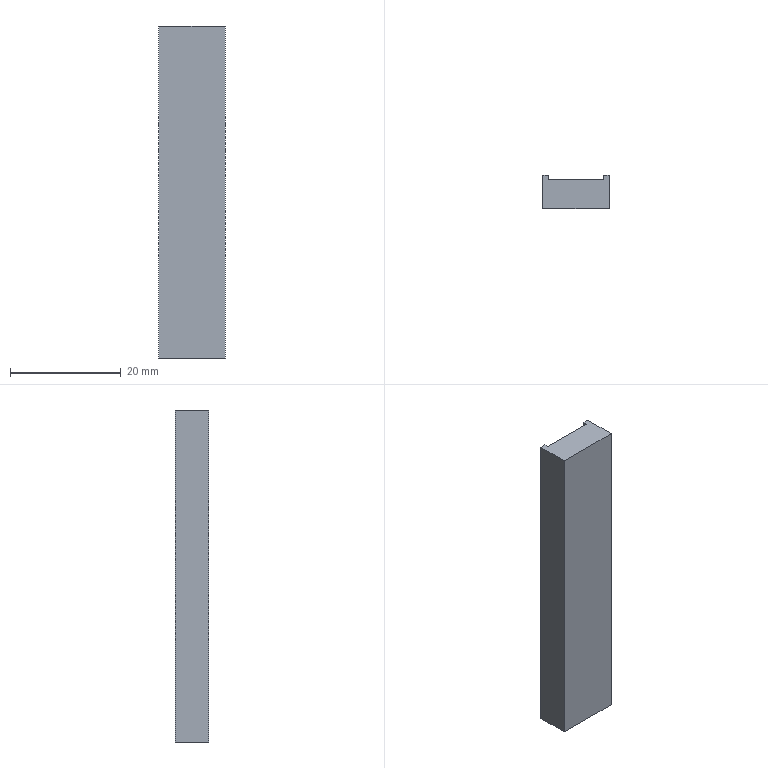Part | SolidWorks | features Extrusion 1, ICE 1 | 1 solid | 10 faces | box 12 x 6 x 60 mm | volume 3870 mm3 | plane 10
STEP:
#1=CARTESIAN_POINT('',(-5.,6.,-30.));
#2=VERTEX_POINT('',#1);
#3=CARTESIAN_POINT('',(-5.,6.,30.));
#4=VERTEX_POINT('',#3);
#5=CARTESIAN_POINT('',(-5.,6.,30.));
#6=DIRECTION('',(0.,0.,1.));
#7=VECTOR('',#6,1000.);
#8=LINE('',#5,#7);
#9=EDGE_CURVE('',#2,#4,#8,.T.);
#10=ORIENTED_EDGE('',*,*,#9,.F.);
#11=CARTESIAN_POINT('',(-6.,6.,-30.));
#12=VERTEX_POINT('',#11);
#13=CARTESIAN_POINT('',(6.,6.,-30.));
#14=DIRECTION('',(-1.,0.,0.));
#15=VECTOR('',#14,1000.);
#16=LINE('',#13,#15);
#17=EDGE_CURVE('',#2,#12,#16,.T.);
#18=ORIENTED_EDGE('',*,*,#17,.T.);
#19=CARTESIAN_POINT('',(-6.,6.,30.));
#20=VERTEX_POINT('',#19);
#21=CARTESIAN_POINT('',(-6.,6.,30.));
#22=DIRECTION('',(0.,0.,1.));
#23=VECTOR('',#22,1000.);
#24=LINE('',#21,#23);
#25=EDGE_CURVE('',#12,#20,#24,.T.);
#26=ORIENTED_EDGE('',*,*,#25,.T.);
#27=CARTESIAN_POINT('',(6.,6.,30.));
#28=DIRECTION('',(1.,0.,0.));
#29=VECTOR('',#28,1000.);
#30=LINE('',#27,#29);
#31=EDGE_CURVE('',#20,#4,#30,.T.);
#32=ORIENTED_EDGE('',*,*,#31,.T.);
#33=EDGE_LOOP('',(#10,#18,#26,#32));
#34=FACE_OUTER_BOUND('',#33,.T.);
#35=CARTESIAN_POINT('',(0.,6.,0.));
#36=DIRECTION('',(0.,1.,0.));
#37=DIRECTION('',(0.,0.,1.));
#38=AXIS2_PLACEMENT_3D('',#35,#36,#37);
#39=PLANE('',#38);
#40=ADVANCED_FACE('',(#34),#39,.T.);
#41=CARTESIAN_POINT('',(-6.,0.,-30.));
#42=VERTEX_POINT('',#41);
#43=CARTESIAN_POINT('',(-6.,0.,30.));
#44=VERTEX_POINT('',#43);
#45=CARTESIAN_POINT('',(-6.,0.,30.));
#46=DIRECTION('',(0.,0.,1.));
#47=VECTOR('',#46,1000.);
#48=LINE('',#45,#47);
#49=EDGE_CURVE('',#42,#44,#48,.T.);
#50=ORIENTED_EDGE('',*,*,#49,.T.);
#51=CARTESIAN_POINT('',(-6.,6.,30.));
#52=DIRECTION('',(0.,-1.,0.));
#53=VECTOR('',#52,1000.);
#54=LINE('',#51,#53);
#55=EDGE_CURVE('',#20,#44,#54,.T.);
#56=ORIENTED_EDGE('',*,*,#55,.F.);
#57=ORIENTED_EDGE('',*,*,#25,.F.);
#58=CARTESIAN_POINT('',(-6.,6.,-30.));
#59=DIRECTION('',(0.,-1.,0.));
#60=VECTOR('',#59,1000.);
#61=LINE('',#58,#60);
#62=EDGE_CURVE('',#12,#42,#61,.T.);
#63=ORIENTED_EDGE('',*,*,#62,.T.);
#64=EDGE_LOOP('',(#50,#56,#57,#63));
#65=FACE_OUTER_BOUND('',#64,.T.);
#66=CARTESIAN_POINT('',(-6.,6.,30.));
#67=DIRECTION('',(1.,0.,0.));
#68=DIRECTION('',(0.,0.,-1.));
#69=AXIS2_PLACEMENT_3D('',#66,#67,#68);
#70=PLANE('',#69);
#71=ADVANCED_FACE('',(#65),#70,.F.);
#72=CARTESIAN_POINT('',(-5.,5.25,30.));
#73=VERTEX_POINT('',#72);
#74=CARTESIAN_POINT('',(5.,5.25,30.));
#75=VERTEX_POINT('',#74);
#76=CARTESIAN_POINT('',(5.,5.25,30.));
#77=DIRECTION('',(1.,0.,0.));
#78=VECTOR('',#77,1000.);
#79=LINE('',#76,#78);
#80=EDGE_CURVE('',#73,#75,#79,.T.);
#81=ORIENTED_EDGE('',*,*,#80,.F.);
#82=CARTESIAN_POINT('',(-5.,5.25,30.));
#83=DIRECTION('',(0.,1.,0.));
#84=VECTOR('',#83,1000.);
#85=LINE('',#82,#84);
#86=EDGE_CURVE('',#73,#4,#85,.T.);
#87=ORIENTED_EDGE('',*,*,#86,.T.);
#88=ORIENTED_EDGE('',*,*,#31,.F.);
#89=ORIENTED_EDGE('',*,*,#55,.T.);
#90=CARTESIAN_POINT('',(6.,0.,30.));
#91=VERTEX_POINT('',#90);
#92=CARTESIAN_POINT('',(6.,0.,30.));
#93=DIRECTION('',(1.,0.,0.));
#94=VECTOR('',#93,1000.);
#95=LINE('',#92,#94);
#96=EDGE_CURVE('',#44,#91,#95,.T.);
#97=ORIENTED_EDGE('',*,*,#96,.T.);
#98=CARTESIAN_POINT('',(6.,6.,30.));
#99=VERTEX_POINT('',#98);
#100=CARTESIAN_POINT('',(6.,6.,30.));
#101=DIRECTION('',(0.,-1.,0.));
#102=VECTOR('',#101,1000.);
#103=LINE('',#100,#102);
#104=EDGE_CURVE('',#99,#91,#103,.T.);
#105=ORIENTED_EDGE('',*,*,#104,.F.);
#106=CARTESIAN_POINT('',(5.,6.,30.));
#107=VERTEX_POINT('',#106);
#108=CARTESIAN_POINT('',(6.,6.,30.));
#109=DIRECTION('',(1.,0.,0.));
#110=VECTOR('',#109,1000.);
#111=LINE('',#108,#110);
#112=EDGE_CURVE('',#107,#99,#111,.T.);
#113=ORIENTED_EDGE('',*,*,#112,.F.);
#114=CARTESIAN_POINT('',(5.,5.25,30.));
#115=DIRECTION('',(0.,1.,0.));
#116=VECTOR('',#115,1000.);
#117=LINE('',#114,#116);
#118=EDGE_CURVE('',#75,#107,#117,.T.);
#119=ORIENTED_EDGE('',*,*,#118,.F.);
#120=EDGE_LOOP('',(#81,#87,#88,#89,#97,#105,#113,#119));
#121=FACE_OUTER_BOUND('',#120,.T.);
#122=CARTESIAN_POINT('',(6.,6.,30.));
#123=DIRECTION('',(0.,0.,-1.));
#124=DIRECTION('',(-1.,0.,0.));
#125=AXIS2_PLACEMENT_3D('',#122,#123,#124);
#126=PLANE('',#125);
#127=ADVANCED_FACE('',(#121),#126,.F.);
#128=CARTESIAN_POINT('',(6.,0.,-30.));
#129=VERTEX_POINT('',#128);
#130=CARTESIAN_POINT('',(6.,0.,30.));
#131=DIRECTION('',(0.,0.,-1.));
#132=VECTOR('',#131,1000.);
#133=LINE('',#130,#132);
#134=EDGE_CURVE('',#91,#129,#133,.T.);
#135=ORIENTED_EDGE('',*,*,#134,.T.);
#136=CARTESIAN_POINT('',(6.,6.,-30.));
#137=VERTEX_POINT('',#136);
#138=CARTESIAN_POINT('',(6.,6.,-30.));
#139=DIRECTION('',(0.,-1.,0.));
#140=VECTOR('',#139,1000.);
#141=LINE('',#138,#140);
#142=EDGE_CURVE('',#137,#129,#141,.T.);
#143=ORIENTED_EDGE('',*,*,#142,.F.);
#144=CARTESIAN_POINT('',(6.,6.,30.));
#145=DIRECTION('',(0.,0.,-1.));
#146=VECTOR('',#145,1000.);
#147=LINE('',#144,#146);
#148=EDGE_CURVE('',#99,#137,#147,.T.);
#149=ORIENTED_EDGE('',*,*,#148,.F.);
#150=ORIENTED_EDGE('',*,*,#104,.T.);
#151=EDGE_LOOP('',(#135,#143,#149,#150));
#152=FACE_OUTER_BOUND('',#151,.T.);
#153=CARTESIAN_POINT('',(6.,6.,30.));
#154=DIRECTION('',(-1.,0.,0.));
#155=DIRECTION('',(0.,0.,1.));
#156=AXIS2_PLACEMENT_3D('',#153,#154,#155);
#157=PLANE('',#156);
#158=ADVANCED_FACE('',(#152),#157,.F.);
#159=ORIENTED_EDGE('',*,*,#17,.F.);
#160=CARTESIAN_POINT('',(-5.,5.25,-30.));
#161=VERTEX_POINT('',#160);
#162=CARTESIAN_POINT('',(-5.,5.25,-30.));
#163=DIRECTION('',(0.,1.,0.));
#164=VECTOR('',#163,1000.);
#165=LINE('',#162,#164);
#166=EDGE_CURVE('',#161,#2,#165,.T.);
#167=ORIENTED_EDGE('',*,*,#166,.F.);
#168=CARTESIAN_POINT('',(5.,5.25,-30.));
#169=VERTEX_POINT('',#168);
#170=CARTESIAN_POINT('',(5.,5.25,-30.));
#171=DIRECTION('',(-1.,0.,0.));
#172=VECTOR('',#171,1000.);
#173=LINE('',#170,#172);
#174=EDGE_CURVE('',#169,#161,#173,.T.);
#175=ORIENTED_EDGE('',*,*,#174,.F.);
#176=CARTESIAN_POINT('',(5.,6.,-30.));
#177=VERTEX_POINT('',#176);
#178=CARTESIAN_POINT('',(5.,5.25,-30.));
#179=DIRECTION('',(0.,1.,0.));
#180=VECTOR('',#179,1000.);
#181=LINE('',#178,#180);
#182=EDGE_CURVE('',#169,#177,#181,.T.);
#183=ORIENTED_EDGE('',*,*,#182,.T.);
#184=CARTESIAN_POINT('',(6.,6.,-30.));
#185=DIRECTION('',(-1.,0.,0.));
#186=VECTOR('',#185,1000.);
#187=LINE('',#184,#186);
#188=EDGE_CURVE('',#137,#177,#187,.T.);
#189=ORIENTED_EDGE('',*,*,#188,.F.);
#190=ORIENTED_EDGE('',*,*,#142,.T.);
#191=CARTESIAN_POINT('',(6.,0.,-30.));
#192=DIRECTION('',(-1.,0.,0.));
#193=VECTOR('',#192,1000.);
#194=LINE('',#191,#193);
#195=EDGE_CURVE('',#129,#42,#194,.T.);
#196=ORIENTED_EDGE('',*,*,#195,.T.);
#197=ORIENTED_EDGE('',*,*,#62,.F.);
#198=EDGE_LOOP('',(#159,#167,#175,#183,#189,#190,#196,#197));
#199=FACE_OUTER_BOUND('',#198,.T.);
#200=CARTESIAN_POINT('',(6.,6.,-30.));
#201=DIRECTION('',(0.,0.,1.));
#202=DIRECTION('',(1.,0.,0.));
#203=AXIS2_PLACEMENT_3D('',#200,#201,#202);
#204=PLANE('',#203);
#205=ADVANCED_FACE('',(#199),#204,.F.);
#206=CARTESIAN_POINT('',(5.,6.,30.));
#207=DIRECTION('',(0.,0.,-1.));
#208=VECTOR('',#207,1000.);
#209=LINE('',#206,#208);
#210=EDGE_CURVE('',#107,#177,#209,.T.);
#211=ORIENTED_EDGE('',*,*,#210,.F.);
#212=ORIENTED_EDGE('',*,*,#112,.T.);
#213=ORIENTED_EDGE('',*,*,#148,.T.);
#214=ORIENTED_EDGE('',*,*,#188,.T.);
#215=EDGE_LOOP('',(#211,#212,#213,#214));
#216=FACE_OUTER_BOUND('',#215,.T.);
#217=CARTESIAN_POINT('',(0.,6.,0.));
#218=DIRECTION('',(0.,1.,0.));
#219=DIRECTION('',(0.,0.,1.));
#220=AXIS2_PLACEMENT_3D('',#217,#218,#219);
#221=PLANE('',#220);
#222=ADVANCED_FACE('',(#216),#221,.T.);
#223=ORIENTED_EDGE('',*,*,#49,.F.);
#224=ORIENTED_EDGE('',*,*,#195,.F.);
#225=ORIENTED_EDGE('',*,*,#134,.F.);
#226=ORIENTED_EDGE('',*,*,#96,.F.);
#227=EDGE_LOOP('',(#223,#224,#225,#226));
#228=FACE_OUTER_BOUND('',#227,.T.);
#229=CARTESIAN_POINT('',(0.,0.,0.));
#230=DIRECTION('',(0.,1.,0.));
#231=DIRECTION('',(0.,0.,1.));
#232=AXIS2_PLACEMENT_3D('',#229,#230,#231);
#233=PLANE('',#232);
#234=ADVANCED_FACE('',(#228),#233,.F.);
#235=ORIENTED_EDGE('',*,*,#9,.T.);
#236=ORIENTED_EDGE('',*,*,#86,.F.);
#237=CARTESIAN_POINT('',(-5.,5.25,30.));
#238=DIRECTION('',(0.,0.,1.));
#239=VECTOR('',#238,1000.);
#240=LINE('',#237,#239);
#241=EDGE_CURVE('',#161,#73,#240,.T.);
#242=ORIENTED_EDGE('',*,*,#241,.F.);
#243=ORIENTED_EDGE('',*,*,#166,.T.);
#244=EDGE_LOOP('',(#235,#236,#242,#243));
#245=FACE_OUTER_BOUND('',#244,.T.);
#246=CARTESIAN_POINT('',(-5.,5.25,30.));
#247=DIRECTION('',(-1.,0.,0.));
#248=DIRECTION('',(0.,0.,1.));
#249=AXIS2_PLACEMENT_3D('',#246,#247,#248);
#250=PLANE('',#249);
#251=ADVANCED_FACE('',(#245),#250,.F.);
#252=ORIENTED_EDGE('',*,*,#210,.T.);
#253=ORIENTED_EDGE('',*,*,#182,.F.);
#254=CARTESIAN_POINT('',(5.,5.25,30.));
#255=DIRECTION('',(0.,0.,-1.));
#256=VECTOR('',#255,1000.);
#257=LINE('',#254,#256);
#258=EDGE_CURVE('',#75,#169,#257,.T.);
#259=ORIENTED_EDGE('',*,*,#258,.F.);
#260=ORIENTED_EDGE('',*,*,#118,.T.);
#261=EDGE_LOOP('',(#252,#253,#259,#260));
#262=FACE_OUTER_BOUND('',#261,.T.);
#263=CARTESIAN_POINT('',(5.,5.25,30.));
#264=DIRECTION('',(1.,0.,0.));
#265=DIRECTION('',(0.,0.,-1.));
#266=AXIS2_PLACEMENT_3D('',#263,#264,#265);
#267=PLANE('',#266);
#268=ADVANCED_FACE('',(#262),#267,.F.);
#269=ORIENTED_EDGE('',*,*,#241,.T.);
#270=ORIENTED_EDGE('',*,*,#80,.T.);
#271=ORIENTED_EDGE('',*,*,#258,.T.);
#272=ORIENTED_EDGE('',*,*,#174,.T.);
#273=EDGE_LOOP('',(#269,#270,#271,#272));
#274=FACE_OUTER_BOUND('',#273,.T.);
#275=CARTESIAN_POINT('',(0.,5.25,0.));
#276=DIRECTION('',(0.,1.,0.));
#277=DIRECTION('',(0.,0.,1.));
#278=AXIS2_PLACEMENT_3D('',#275,#276,#277);
#279=PLANE('',#278);
#280=ADVANCED_FACE('',(#274),#279,.T.);
#281=CLOSED_SHELL('',(#40,#71,#127,#158,#205,#222,#234,#251,#268,#280));
#282=MANIFOLD_SOLID_BREP('',#281);
#283=CARTESIAN_POINT('',(0.,0.,0.));
#284=DIRECTION('',(0.,0.,1.));
#285=DIRECTION('',(1.,0.,0.));
#286=AXIS2_PLACEMENT_3D('',#283,#284,#285);
#287=(LENGTH_UNIT()NAMED_UNIT(*)SI_UNIT(.MILLI.,.METRE.));
#288=UNCERTAINTY_MEASURE_WITH_UNIT(LENGTH_MEASURE(0.00001),#287,'','');
#289=(NAMED_UNIT(*)PLANE_ANGLE_UNIT()SI_UNIT($,.RADIAN.));
#290=(NAMED_UNIT(*)SI_UNIT($,.STERADIAN.)SOLID_ANGLE_UNIT());
#291=(GEOMETRIC_REPRESENTATION_CONTEXT(3)GLOBAL_UNCERTAINTY_ASSIGNED_CONTEXT((#288))GLOBAL_UNIT_ASSIGNED_CONTEXT((#287,#289,#290))REPRESENTATION_CONTEXT('',''));
#292=ADVANCED_BREP_SHAPE_REPRESENTATION('',(#282,#286),#291);